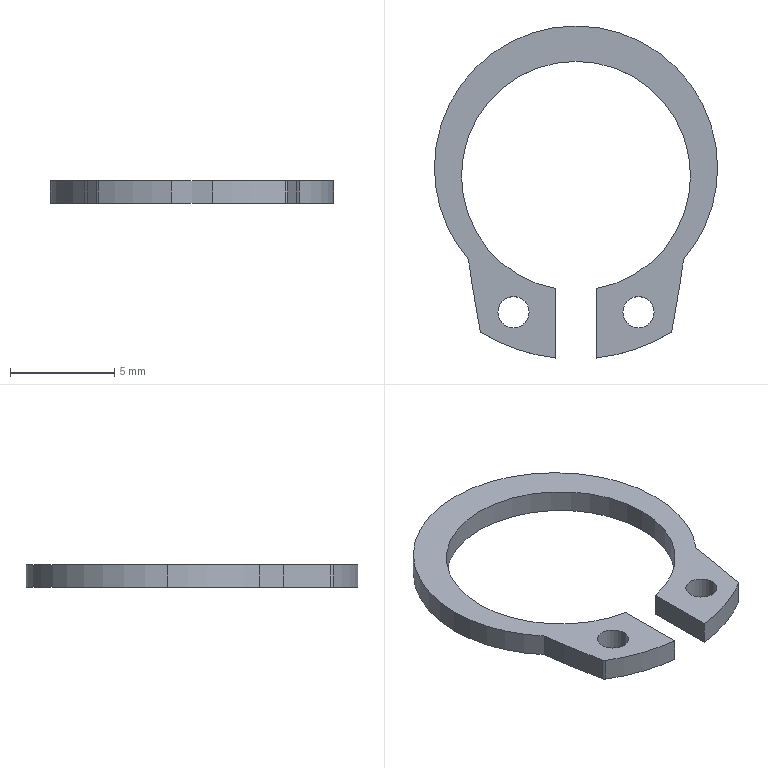Part | SolidWorks | features Extrusion 1 | 1 solid | 22 faces | box 13.6 x 15.943 x 1.1 mm | volume 71.659 mm3 | cylinder 14 | plane 8 | commonest cylinder face diameters 1.5 x4 11 x3 13.6 x3 0.4 x2 17.6 x2
STEP:
#1=CARTESIAN_POINT('',(2.25,-6.545,1.1));
#2=VERTEX_POINT('',#1);
#3=CARTESIAN_POINT('',(3.75,-6.545,1.1));
#4=VERTEX_POINT('',#3);
#5=CARTESIAN_POINT('',(3.,-6.545,1.1));
#6=DIRECTION('',(0.,0.,1.));
#7=DIRECTION('',(1.,0.,0.));
#8=AXIS2_PLACEMENT_3D('',#5,#6,#7);
#9=CIRCLE('',#8,0.75);
#10=EDGE_CURVE('',#2,#4,#9,.T.);
#11=ORIENTED_EDGE('',*,*,#10,.T.);
#12=CARTESIAN_POINT('',(3.75,-6.545,0.));
#13=VERTEX_POINT('',#12);
#14=CARTESIAN_POINT('',(3.75,-6.545,1.1));
#15=DIRECTION('',(0.,0.,-1.));
#16=VECTOR('',#15,1000.);
#17=LINE('',#14,#16);
#18=EDGE_CURVE('',#4,#13,#17,.T.);
#19=ORIENTED_EDGE('',*,*,#18,.T.);
#20=CARTESIAN_POINT('',(2.25,-6.545,0.));
#21=VERTEX_POINT('',#20);
#22=CARTESIAN_POINT('',(3.,-6.545,0.));
#23=DIRECTION('',(0.,0.,1.));
#24=DIRECTION('',(1.,0.,0.));
#25=AXIS2_PLACEMENT_3D('',#22,#23,#24);
#26=CIRCLE('',#25,0.75);
#27=EDGE_CURVE('',#21,#13,#26,.T.);
#28=ORIENTED_EDGE('',*,*,#27,.F.);
#29=CARTESIAN_POINT('',(2.25,-6.545,1.1));
#30=DIRECTION('',(0.,0.,-1.));
#31=VECTOR('',#30,1000.);
#32=LINE('',#29,#31);
#33=EDGE_CURVE('',#2,#21,#32,.T.);
#34=ORIENTED_EDGE('',*,*,#33,.F.);
#35=EDGE_LOOP('',(#11,#19,#28,#34));
#36=FACE_OUTER_BOUND('',#35,.T.);
#37=CARTESIAN_POINT('',(3.,-6.545,1.1));
#38=DIRECTION('',(0.,0.,-1.));
#39=DIRECTION('',(-1.,0.,0.));
#40=AXIS2_PLACEMENT_3D('',#37,#38,#39);
#41=CYLINDRICAL_SURFACE('',#40,0.75);
#42=ADVANCED_FACE('',(#36),#41,.F.);
#43=CARTESIAN_POINT('',(-3.75,-6.545,1.1));
#44=VERTEX_POINT('',#43);
#45=CARTESIAN_POINT('',(-2.25,-6.545,1.1));
#46=VERTEX_POINT('',#45);
#47=CARTESIAN_POINT('',(-3.,-6.545,1.1));
#48=DIRECTION('',(0.,0.,1.));
#49=DIRECTION('',(1.,0.,0.));
#50=AXIS2_PLACEMENT_3D('',#47,#48,#49);
#51=CIRCLE('',#50,0.75);
#52=EDGE_CURVE('',#44,#46,#51,.T.);
#53=ORIENTED_EDGE('',*,*,#52,.T.);
#54=CARTESIAN_POINT('',(-2.25,-6.545,0.));
#55=VERTEX_POINT('',#54);
#56=CARTESIAN_POINT('',(-2.25,-6.545,1.1));
#57=DIRECTION('',(0.,0.,-1.));
#58=VECTOR('',#57,1000.);
#59=LINE('',#56,#58);
#60=EDGE_CURVE('',#46,#55,#59,.T.);
#61=ORIENTED_EDGE('',*,*,#60,.T.);
#62=CARTESIAN_POINT('',(-3.75,-6.545,0.));
#63=VERTEX_POINT('',#62);
#64=CARTESIAN_POINT('',(-3.,-6.545,0.));
#65=DIRECTION('',(0.,0.,1.));
#66=DIRECTION('',(1.,0.,0.));
#67=AXIS2_PLACEMENT_3D('',#64,#65,#66);
#68=CIRCLE('',#67,0.75);
#69=EDGE_CURVE('',#63,#55,#68,.T.);
#70=ORIENTED_EDGE('',*,*,#69,.F.);
#71=CARTESIAN_POINT('',(-3.75,-6.545,1.1));
#72=DIRECTION('',(0.,0.,-1.));
#73=VECTOR('',#72,1000.);
#74=LINE('',#71,#73);
#75=EDGE_CURVE('',#44,#63,#74,.T.);
#76=ORIENTED_EDGE('',*,*,#75,.F.);
#77=EDGE_LOOP('',(#53,#61,#70,#76));
#78=FACE_OUTER_BOUND('',#77,.T.);
#79=CARTESIAN_POINT('',(-3.,-6.545,1.1));
#80=DIRECTION('',(0.,0.,-1.));
#81=DIRECTION('',(-1.,0.,0.));
#82=AXIS2_PLACEMENT_3D('',#79,#80,#81);
#83=CYLINDRICAL_SURFACE('',#82,0.75);
#84=ADVANCED_FACE('',(#78),#83,.F.);
#85=CARTESIAN_POINT('',(6.8,0.4,1.1));
#86=VERTEX_POINT('',#85);
#87=CARTESIAN_POINT('',(-6.8,0.4,1.1));
#88=VERTEX_POINT('',#87);
#89=CARTESIAN_POINT('',(0.,0.4,1.1));
#90=DIRECTION('',(0.,0.,1.));
#91=DIRECTION('',(1.,0.,0.));
#92=AXIS2_PLACEMENT_3D('',#89,#90,#91);
#93=CIRCLE('',#92,6.8);
#94=EDGE_CURVE('',#86,#88,#93,.T.);
#95=ORIENTED_EDGE('',*,*,#94,.F.);
#96=CARTESIAN_POINT('',(6.8,0.4,0.));
#97=VERTEX_POINT('',#96);
#98=CARTESIAN_POINT('',(6.8,0.4,1.1));
#99=DIRECTION('',(0.,0.,-1.));
#100=VECTOR('',#99,1000.);
#101=LINE('',#98,#100);
#102=EDGE_CURVE('',#86,#97,#101,.T.);
#103=ORIENTED_EDGE('',*,*,#102,.T.);
#104=CARTESIAN_POINT('',(-6.8,0.4,0.));
#105=VERTEX_POINT('',#104);
#106=CARTESIAN_POINT('',(0.,0.4,0.));
#107=DIRECTION('',(0.,0.,1.));
#108=DIRECTION('',(1.,0.,0.));
#109=AXIS2_PLACEMENT_3D('',#106,#107,#108);
#110=CIRCLE('',#109,6.8);
#111=EDGE_CURVE('',#97,#105,#110,.T.);
#112=ORIENTED_EDGE('',*,*,#111,.T.);
#113=CARTESIAN_POINT('',(-6.8,0.4,1.1));
#114=DIRECTION('',(0.,0.,-1.));
#115=VECTOR('',#114,1000.);
#116=LINE('',#113,#115);
#117=EDGE_CURVE('',#88,#105,#116,.T.);
#118=ORIENTED_EDGE('',*,*,#117,.F.);
#119=EDGE_LOOP('',(#95,#103,#112,#118));
#120=FACE_OUTER_BOUND('',#119,.T.);
#121=CARTESIAN_POINT('',(0.,0.4,1.1));
#122=DIRECTION('',(0.,0.,-1.));
#123=DIRECTION('',(-1.,0.,0.));
#124=AXIS2_PLACEMENT_3D('',#121,#122,#123);
#125=CYLINDRICAL_SURFACE('',#124,6.8);
#126=ADVANCED_FACE('',(#120),#125,.T.);
#127=CARTESIAN_POINT('',(-5.16,-4.028,1.1));
#128=VERTEX_POINT('',#127);
#129=CARTESIAN_POINT('',(0.,0.4,1.1));
#130=DIRECTION('',(0.,0.,1.));
#131=DIRECTION('',(1.,0.,0.));
#132=AXIS2_PLACEMENT_3D('',#129,#130,#131);
#133=CIRCLE('',#132,6.8);
#134=EDGE_CURVE('',#88,#128,#133,.T.);
#135=ORIENTED_EDGE('',*,*,#134,.F.);
#136=ORIENTED_EDGE('',*,*,#117,.T.);
#137=CARTESIAN_POINT('',(-5.16,-4.028,0.));
#138=VERTEX_POINT('',#137);
#139=CARTESIAN_POINT('',(0.,0.4,0.));
#140=DIRECTION('',(0.,0.,1.));
#141=DIRECTION('',(1.,0.,0.));
#142=AXIS2_PLACEMENT_3D('',#139,#140,#141);
#143=CIRCLE('',#142,6.8);
#144=EDGE_CURVE('',#105,#138,#143,.T.);
#145=ORIENTED_EDGE('',*,*,#144,.T.);
#146=CARTESIAN_POINT('',(-5.16,-4.028,1.1));
#147=DIRECTION('',(0.,0.,-1.));
#148=VECTOR('',#147,1000.);
#149=LINE('',#146,#148);
#150=EDGE_CURVE('',#128,#138,#149,.T.);
#151=ORIENTED_EDGE('',*,*,#150,.F.);
#152=EDGE_LOOP('',(#135,#136,#145,#151));
#153=FACE_OUTER_BOUND('',#152,.T.);
#154=CARTESIAN_POINT('',(0.,0.4,1.1));
#155=DIRECTION('',(0.,0.,-1.));
#156=DIRECTION('',(-1.,0.,0.));
#157=AXIS2_PLACEMENT_3D('',#154,#155,#156);
#158=CYLINDRICAL_SURFACE('',#157,6.8);
#159=ADVANCED_FACE('',(#153),#158,.T.);
#160=CARTESIAN_POINT('',(1.,-5.408,1.1));
#161=VERTEX_POINT('',#160);
#162=CARTESIAN_POINT('',(5.5,0.,1.1));
#163=VERTEX_POINT('',#162);
#164=CARTESIAN_POINT('',(0.,0.,1.1));
#165=DIRECTION('',(0.,0.,1.));
#166=DIRECTION('',(1.,0.,0.));
#167=AXIS2_PLACEMENT_3D('',#164,#165,#166);
#168=CIRCLE('',#167,5.5);
#169=EDGE_CURVE('',#161,#163,#168,.T.);
#170=ORIENTED_EDGE('',*,*,#169,.T.);
#171=CARTESIAN_POINT('',(5.5,0.,0.));
#172=VERTEX_POINT('',#171);
#173=CARTESIAN_POINT('',(5.5,0.,1.1));
#174=DIRECTION('',(0.,0.,-1.));
#175=VECTOR('',#174,1000.);
#176=LINE('',#173,#175);
#177=EDGE_CURVE('',#163,#172,#176,.T.);
#178=ORIENTED_EDGE('',*,*,#177,.T.);
#179=CARTESIAN_POINT('',(1.,-5.408,0.));
#180=VERTEX_POINT('',#179);
#181=CARTESIAN_POINT('',(0.,0.,0.));
#182=DIRECTION('',(0.,0.,1.));
#183=DIRECTION('',(1.,0.,0.));
#184=AXIS2_PLACEMENT_3D('',#181,#182,#183);
#185=CIRCLE('',#184,5.5);
#186=EDGE_CURVE('',#180,#172,#185,.T.);
#187=ORIENTED_EDGE('',*,*,#186,.F.);
#188=CARTESIAN_POINT('',(1.,-5.408,1.1));
#189=DIRECTION('',(0.,0.,-1.));
#190=VECTOR('',#189,1000.);
#191=LINE('',#188,#190);
#192=EDGE_CURVE('',#161,#180,#191,.T.);
#193=ORIENTED_EDGE('',*,*,#192,.F.);
#194=EDGE_LOOP('',(#170,#178,#187,#193));
#195=FACE_OUTER_BOUND('',#194,.T.);
#196=CARTESIAN_POINT('',(0.,0.,1.1));
#197=DIRECTION('',(0.,0.,-1.));
#198=DIRECTION('',(-1.,0.,0.));
#199=AXIS2_PLACEMENT_3D('',#196,#197,#198);
#200=CYLINDRICAL_SURFACE('',#199,5.5);
#201=ADVANCED_FACE('',(#195),#200,.F.);
#202=ORIENTED_EDGE('',*,*,#177,.F.);
#203=CARTESIAN_POINT('',(-5.5,0.,1.1));
#204=VERTEX_POINT('',#203);
#205=CARTESIAN_POINT('',(0.,0.,1.1));
#206=DIRECTION('',(0.,0.,1.));
#207=DIRECTION('',(1.,0.,0.));
#208=AXIS2_PLACEMENT_3D('',#205,#206,#207);
#209=CIRCLE('',#208,5.5);
#210=EDGE_CURVE('',#163,#204,#209,.T.);
#211=ORIENTED_EDGE('',*,*,#210,.T.);
#212=CARTESIAN_POINT('',(-5.5,0.,0.));
#213=VERTEX_POINT('',#212);
#214=CARTESIAN_POINT('',(-5.5,0.,1.1));
#215=DIRECTION('',(0.,0.,-1.));
#216=VECTOR('',#215,1000.);
#217=LINE('',#214,#216);
#218=EDGE_CURVE('',#204,#213,#217,.T.);
#219=ORIENTED_EDGE('',*,*,#218,.T.);
#220=CARTESIAN_POINT('',(0.,0.,0.));
#221=DIRECTION('',(0.,0.,1.));
#222=DIRECTION('',(1.,0.,0.));
#223=AXIS2_PLACEMENT_3D('',#220,#221,#222);
#224=CIRCLE('',#223,5.5);
#225=EDGE_CURVE('',#172,#213,#224,.T.);
#226=ORIENTED_EDGE('',*,*,#225,.F.);
#227=EDGE_LOOP('',(#202,#211,#219,#226));
#228=FACE_OUTER_BOUND('',#227,.T.);
#229=CARTESIAN_POINT('',(0.,0.,1.1));
#230=DIRECTION('',(0.,0.,-1.));
#231=DIRECTION('',(-1.,0.,0.));
#232=AXIS2_PLACEMENT_3D('',#229,#230,#231);
#233=CYLINDRICAL_SURFACE('',#232,5.5);
#234=ADVANCED_FACE('',(#228),#233,.F.);
#235=CARTESIAN_POINT('',(-4.511,-7.556,0.));
#236=VERTEX_POINT('',#235);
#237=CARTESIAN_POINT('',(-4.605,-7.419,0.));
#238=VERTEX_POINT('',#237);
#239=CARTESIAN_POINT('',(-4.408,-7.384,0.));
#240=DIRECTION('',(0.,0.,-1.));
#241=DIRECTION('',(1.,0.,0.));
#242=AXIS2_PLACEMENT_3D('',#239,#240,#241);
#243=CIRCLE('',#242,0.2);
#244=EDGE_CURVE('',#236,#238,#243,.T.);
#245=ORIENTED_EDGE('',*,*,#244,.F.);
#246=CARTESIAN_POINT('',(-4.511,-7.556,1.1));
#247=VERTEX_POINT('',#246);
#248=CARTESIAN_POINT('',(-4.511,-7.556,1.1));
#249=DIRECTION('',(0.,0.,-1.));
#250=VECTOR('',#249,1000.);
#251=LINE('',#248,#250);
#252=EDGE_CURVE('',#247,#236,#251,.T.);
#253=ORIENTED_EDGE('',*,*,#252,.F.);
#254=CARTESIAN_POINT('',(-4.605,-7.419,1.1));
#255=VERTEX_POINT('',#254);
#256=CARTESIAN_POINT('',(-4.408,-7.384,1.1));
#257=DIRECTION('',(0.,0.,-1.));
#258=DIRECTION('',(1.,0.,0.));
#259=AXIS2_PLACEMENT_3D('',#256,#257,#258);
#260=CIRCLE('',#259,0.2);
#261=EDGE_CURVE('',#247,#255,#260,.T.);
#262=ORIENTED_EDGE('',*,*,#261,.T.);
#263=CARTESIAN_POINT('',(-4.605,-7.419,1.1));
#264=DIRECTION('',(0.,0.,-1.));
#265=VECTOR('',#264,1000.);
#266=LINE('',#263,#265);
#267=EDGE_CURVE('',#255,#238,#266,.T.);
#268=ORIENTED_EDGE('',*,*,#267,.T.);
#269=EDGE_LOOP('',(#245,#253,#262,#268));
#270=FACE_OUTER_BOUND('',#269,.T.);
#271=CARTESIAN_POINT('',(-4.408,-7.384,1.1));
#272=DIRECTION('',(0.,0.,-1.));
#273=DIRECTION('',(-1.,0.,0.));
#274=AXIS2_PLACEMENT_3D('',#271,#272,#273);
#275=CYLINDRICAL_SURFACE('',#274,0.2);
#276=ADVANCED_FACE('',(#270),#275,.T.);
#277=CARTESIAN_POINT('',(-1.,-8.743,0.));
#278=VERTEX_POINT('',#277);
#279=CARTESIAN_POINT('',(0.,0.,0.));
#280=DIRECTION('',(0.,0.,1.));
#281=DIRECTION('',(1.,0.,0.));
#282=AXIS2_PLACEMENT_3D('',#279,#280,#281);
#283=CIRCLE('',#282,8.8);
#284=EDGE_CURVE('',#236,#278,#283,.T.);
#285=ORIENTED_EDGE('',*,*,#284,.T.);
#286=CARTESIAN_POINT('',(-1.,-8.743,1.1));
#287=VERTEX_POINT('',#286);
#288=CARTESIAN_POINT('',(-1.,-8.743,1.1));
#289=DIRECTION('',(0.,0.,-1.));
#290=VECTOR('',#289,1000.);
#291=LINE('',#288,#290);
#292=EDGE_CURVE('',#287,#278,#291,.T.);
#293=ORIENTED_EDGE('',*,*,#292,.F.);
#294=CARTESIAN_POINT('',(0.,0.,1.1));
#295=DIRECTION('',(0.,0.,1.));
#296=DIRECTION('',(1.,0.,0.));
#297=AXIS2_PLACEMENT_3D('',#294,#295,#296);
#298=CIRCLE('',#297,8.8);
#299=EDGE_CURVE('',#247,#287,#298,.T.);
#300=ORIENTED_EDGE('',*,*,#299,.F.);
#301=ORIENTED_EDGE('',*,*,#252,.T.);
#302=EDGE_LOOP('',(#285,#293,#300,#301));
#303=FACE_OUTER_BOUND('',#302,.T.);
#304=CARTESIAN_POINT('',(0.,0.,1.1));
#305=DIRECTION('',(0.,0.,-1.));
#306=DIRECTION('',(-1.,0.,0.));
#307=AXIS2_PLACEMENT_3D('',#304,#305,#306);
#308=CYLINDRICAL_SURFACE('',#307,8.8);
#309=ADVANCED_FACE('',(#303),#308,.T.);
#310=CARTESIAN_POINT('',(-1.,-5.408,0.));
#311=VERTEX_POINT('',#310);
#312=CARTESIAN_POINT('',(-1.,0.,0.));
#313=DIRECTION('',(0.,-1.,0.));
#314=VECTOR('',#313,1000.);
#315=LINE('',#312,#314);
#316=EDGE_CURVE('',#311,#278,#315,.T.);
#317=ORIENTED_EDGE('',*,*,#316,.F.);
#318=CARTESIAN_POINT('',(-1.,-5.408,1.1));
#319=VERTEX_POINT('',#318);
#320=CARTESIAN_POINT('',(-1.,-5.408,1.1));
#321=DIRECTION('',(0.,0.,-1.));
#322=VECTOR('',#321,1000.);
#323=LINE('',#320,#322);
#324=EDGE_CURVE('',#319,#311,#323,.T.);
#325=ORIENTED_EDGE('',*,*,#324,.F.);
#326=CARTESIAN_POINT('',(-1.,0.,1.1));
#327=DIRECTION('',(0.,-1.,0.));
#328=VECTOR('',#327,1000.);
#329=LINE('',#326,#328);
#330=EDGE_CURVE('',#319,#287,#329,.T.);
#331=ORIENTED_EDGE('',*,*,#330,.T.);
#332=ORIENTED_EDGE('',*,*,#292,.T.);
#333=EDGE_LOOP('',(#317,#325,#331,#332));
#334=FACE_OUTER_BOUND('',#333,.T.);
#335=CARTESIAN_POINT('',(-1.,0.,1.1));
#336=DIRECTION('',(1.,0.,0.));
#337=DIRECTION('',(0.,1.,0.));
#338=AXIS2_PLACEMENT_3D('',#335,#336,#337);
#339=PLANE('',#338);
#340=ADVANCED_FACE('',(#334),#339,.T.);
#341=ORIENTED_EDGE('',*,*,#218,.F.);
#342=CARTESIAN_POINT('',(0.,0.,1.1));
#343=DIRECTION('',(0.,0.,1.));
#344=DIRECTION('',(1.,0.,0.));
#345=AXIS2_PLACEMENT_3D('',#342,#343,#344);
#346=CIRCLE('',#345,5.5);
#347=EDGE_CURVE('',#204,#319,#346,.T.);
#348=ORIENTED_EDGE('',*,*,#347,.T.);
#349=ORIENTED_EDGE('',*,*,#324,.T.);
#350=CARTESIAN_POINT('',(0.,0.,0.));
#351=DIRECTION('',(0.,0.,1.));
#352=DIRECTION('',(1.,0.,0.));
#353=AXIS2_PLACEMENT_3D('',#350,#351,#352);
#354=CIRCLE('',#353,5.5);
#355=EDGE_CURVE('',#213,#311,#354,.T.);
#356=ORIENTED_EDGE('',*,*,#355,.F.);
#357=EDGE_LOOP('',(#341,#348,#349,#356));
#358=FACE_OUTER_BOUND('',#357,.T.);
#359=CARTESIAN_POINT('',(0.,0.,1.1));
#360=DIRECTION('',(0.,0.,-1.));
#361=DIRECTION('',(-1.,0.,0.));
#362=AXIS2_PLACEMENT_3D('',#359,#360,#361);
#363=CYLINDRICAL_SURFACE('',#362,5.5);
#364=ADVANCED_FACE('',(#358),#363,.F.);
#365=CARTESIAN_POINT('',(1.,-8.743,0.));
#366=VERTEX_POINT('',#365);
#367=CARTESIAN_POINT('',(1.,0.,0.));
#368=DIRECTION('',(0.,1.,0.));
#369=VECTOR('',#368,1000.);
#370=LINE('',#367,#369);
#371=EDGE_CURVE('',#366,#180,#370,.T.);
#372=ORIENTED_EDGE('',*,*,#371,.F.);
#373=CARTESIAN_POINT('',(1.,-8.743,1.1));
#374=VERTEX_POINT('',#373);
#375=CARTESIAN_POINT('',(1.,-8.743,1.1));
#376=DIRECTION('',(0.,0.,-1.));
#377=VECTOR('',#376,1000.);
#378=LINE('',#375,#377);
#379=EDGE_CURVE('',#374,#366,#378,.T.);
#380=ORIENTED_EDGE('',*,*,#379,.F.);
#381=CARTESIAN_POINT('',(1.,0.,1.1));
#382=DIRECTION('',(0.,1.,0.));
#383=VECTOR('',#382,1000.);
#384=LINE('',#381,#383);
#385=EDGE_CURVE('',#374,#161,#384,.T.);
#386=ORIENTED_EDGE('',*,*,#385,.T.);
#387=ORIENTED_EDGE('',*,*,#192,.T.);
#388=EDGE_LOOP('',(#372,#380,#386,#387));
#389=FACE_OUTER_BOUND('',#388,.T.);
#390=CARTESIAN_POINT('',(1.,0.,1.1));
#391=DIRECTION('',(-1.,0.,0.));
#392=DIRECTION('',(0.,0.,1.));
#393=AXIS2_PLACEMENT_3D('',#390,#391,#392);
#394=PLANE('',#393);
#395=ADVANCED_FACE('',(#389),#394,.T.);
#396=CARTESIAN_POINT('',(4.511,-7.556,0.));
#397=VERTEX_POINT('',#396);
#398=CARTESIAN_POINT('',(0.,0.,0.));
#399=DIRECTION('',(0.,0.,1.));
#400=DIRECTION('',(1.,0.,0.));
#401=AXIS2_PLACEMENT_3D('',#398,#399,#400);
#402=CIRCLE('',#401,8.8);
#403=EDGE_CURVE('',#366,#397,#402,.T.);
#404=ORIENTED_EDGE('',*,*,#403,.T.);
#405=CARTESIAN_POINT('',(4.511,-7.556,1.1));
#406=VERTEX_POINT('',#405);
#407=CARTESIAN_POINT('',(4.511,-7.556,1.1));
#408=DIRECTION('',(0.,0.,-1.));
#409=VECTOR('',#408,1000.);
#410=LINE('',#407,#409);
#411=EDGE_CURVE('',#406,#397,#410,.T.);
#412=ORIENTED_EDGE('',*,*,#411,.F.);
#413=CARTESIAN_POINT('',(0.,0.,1.1));
#414=DIRECTION('',(0.,0.,1.));
#415=DIRECTION('',(1.,0.,0.));
#416=AXIS2_PLACEMENT_3D('',#413,#414,#415);
#417=CIRCLE('',#416,8.8);
#418=EDGE_CURVE('',#374,#406,#417,.T.);
#419=ORIENTED_EDGE('',*,*,#418,.F.);
#420=ORIENTED_EDGE('',*,*,#379,.T.);
#421=EDGE_LOOP('',(#404,#412,#419,#420));
#422=FACE_OUTER_BOUND('',#421,.T.);
#423=CARTESIAN_POINT('',(0.,0.,1.1));
#424=DIRECTION('',(0.,0.,-1.));
#425=DIRECTION('',(-1.,0.,0.));
#426=AXIS2_PLACEMENT_3D('',#423,#424,#425);
#427=CYLINDRICAL_SURFACE('',#426,8.8);
#428=ADVANCED_FACE('',(#422),#427,.T.);
#429=CARTESIAN_POINT('',(4.605,-7.419,0.));
#430=VERTEX_POINT('',#429);
#431=CARTESIAN_POINT('',(4.408,-7.384,0.));
#432=DIRECTION('',(0.,0.,1.));
#433=DIRECTION('',(1.,0.,0.));
#434=AXIS2_PLACEMENT_3D('',#431,#432,#433);
#435=CIRCLE('',#434,0.2);
#436=EDGE_CURVE('',#397,#430,#435,.T.);
#437=ORIENTED_EDGE('',*,*,#436,.T.);
#438=CARTESIAN_POINT('',(4.605,-7.419,1.1));
#439=VERTEX_POINT('',#438);
#440=CARTESIAN_POINT('',(4.605,-7.419,1.1));
#441=DIRECTION('',(0.,0.,-1.));
#442=VECTOR('',#441,1000.);
#443=LINE('',#440,#442);
#444=EDGE_CURVE('',#439,#430,#443,.T.);
#445=ORIENTED_EDGE('',*,*,#444,.F.);
#446=CARTESIAN_POINT('',(4.408,-7.384,1.1));
#447=DIRECTION('',(0.,0.,1.));
#448=DIRECTION('',(1.,0.,0.));
#449=AXIS2_PLACEMENT_3D('',#446,#447,#448);
#450=CIRCLE('',#449,0.2);
#451=EDGE_CURVE('',#406,#439,#450,.T.);
#452=ORIENTED_EDGE('',*,*,#451,.F.);
#453=ORIENTED_EDGE('',*,*,#411,.T.);
#454=EDGE_LOOP('',(#437,#445,#452,#453));
#455=FACE_OUTER_BOUND('',#454,.T.);
#456=CARTESIAN_POINT('',(4.408,-7.384,1.1));
#457=DIRECTION('',(0.,0.,-1.));
#458=DIRECTION('',(-1.,0.,0.));
#459=AXIS2_PLACEMENT_3D('',#456,#457,#458);
#460=CYLINDRICAL_SURFACE('',#459,0.2);
#461=ADVANCED_FACE('',(#455),#460,.T.);
#462=CARTESIAN_POINT('',(5.,-5.181,0.));
#463=VERTEX_POINT('',#462);
#464=CARTESIAN_POINT('',(5.735,-1.011,0.));
#465=DIRECTION('',(-0.1736,-0.9848,0.));
#466=VECTOR('',#465,1000.);
#467=LINE('',#464,#466);
#468=EDGE_CURVE('',#463,#430,#467,.T.);
#469=ORIENTED_EDGE('',*,*,#468,.F.);
#470=CARTESIAN_POINT('',(5.,-5.181,1.1));
#471=VERTEX_POINT('',#470);
#472=CARTESIAN_POINT('',(5.,-5.181,1.1));
#473=DIRECTION('',(0.,0.,-1.));
#474=VECTOR('',#473,1000.);
#475=LINE('',#472,#474);
#476=EDGE_CURVE('',#471,#463,#475,.T.);
#477=ORIENTED_EDGE('',*,*,#476,.F.);
#478=CARTESIAN_POINT('',(5.735,-1.011,1.1));
#479=DIRECTION('',(-0.1736,-0.9848,0.));
#480=VECTOR('',#479,1000.);
#481=LINE('',#478,#480);
#482=EDGE_CURVE('',#471,#439,#481,.T.);
#483=ORIENTED_EDGE('',*,*,#482,.T.);
#484=ORIENTED_EDGE('',*,*,#444,.T.);
#485=EDGE_LOOP('',(#469,#477,#483,#484));
#486=FACE_OUTER_BOUND('',#485,.T.);
#487=CARTESIAN_POINT('',(5.735,-1.011,1.1));
#488=DIRECTION('',(0.9848,-0.1736,0.));
#489=DIRECTION('',(0.1736,0.9848,0.));
#490=AXIS2_PLACEMENT_3D('',#487,#488,#489);
#491=PLANE('',#490);
#492=ADVANCED_FACE('',(#486),#491,.T.);
#493=CARTESIAN_POINT('',(5.16,-4.028,0.));
#494=VERTEX_POINT('',#493);
#495=CARTESIAN_POINT('',(5.613,-0.7814,0.));
#496=DIRECTION('',(0.1379,0.9904,0.));
#497=VECTOR('',#496,1000.);
#498=LINE('',#495,#497);
#499=EDGE_CURVE('',#463,#494,#498,.T.);
#500=ORIENTED_EDGE('',*,*,#499,.T.);
#501=CARTESIAN_POINT('',(5.16,-4.028,1.1));
#502=VERTEX_POINT('',#501);
#503=CARTESIAN_POINT('',(5.16,-4.028,1.1));
#504=DIRECTION('',(0.,0.,-1.));
#505=VECTOR('',#504,1000.);
#506=LINE('',#503,#505);
#507=EDGE_CURVE('',#502,#494,#506,.T.);
#508=ORIENTED_EDGE('',*,*,#507,.F.);
#509=CARTESIAN_POINT('',(5.613,-0.7814,1.1));
#510=DIRECTION('',(0.1379,0.9904,0.));
#511=VECTOR('',#510,1000.);
#512=LINE('',#509,#511);
#513=EDGE_CURVE('',#471,#502,#512,.T.);
#514=ORIENTED_EDGE('',*,*,#513,.F.);
#515=ORIENTED_EDGE('',*,*,#476,.T.);
#516=EDGE_LOOP('',(#500,#508,#514,#515));
#517=FACE_OUTER_BOUND('',#516,.T.);
#518=CARTESIAN_POINT('',(5.613,-0.7814,1.1));
#519=DIRECTION('',(-0.9904,0.1379,0.));
#520=DIRECTION('',(-0.1379,-0.9904,0.));
#521=AXIS2_PLACEMENT_3D('',#518,#519,#520);
#522=PLANE('',#521);
#523=ADVANCED_FACE('',(#517),#522,.F.);
#524=ORIENTED_EDGE('',*,*,#102,.F.);
#525=CARTESIAN_POINT('',(0.,0.4,1.1));
#526=DIRECTION('',(0.,0.,1.));
#527=DIRECTION('',(1.,0.,0.));
#528=AXIS2_PLACEMENT_3D('',#525,#526,#527);
#529=CIRCLE('',#528,6.8);
#530=EDGE_CURVE('',#502,#86,#529,.T.);
#531=ORIENTED_EDGE('',*,*,#530,.F.);
#532=ORIENTED_EDGE('',*,*,#507,.T.);
#533=CARTESIAN_POINT('',(0.,0.4,0.));
#534=DIRECTION('',(0.,0.,1.));
#535=DIRECTION('',(1.,0.,0.));
#536=AXIS2_PLACEMENT_3D('',#533,#534,#535);
#537=CIRCLE('',#536,6.8);
#538=EDGE_CURVE('',#494,#97,#537,.T.);
#539=ORIENTED_EDGE('',*,*,#538,.T.);
#540=EDGE_LOOP('',(#524,#531,#532,#539));
#541=FACE_OUTER_BOUND('',#540,.T.);
#542=CARTESIAN_POINT('',(0.,0.4,1.1));
#543=DIRECTION('',(0.,0.,-1.));
#544=DIRECTION('',(-1.,0.,0.));
#545=AXIS2_PLACEMENT_3D('',#542,#543,#544);
#546=CYLINDRICAL_SURFACE('',#545,6.8);
#547=ADVANCED_FACE('',(#541),#546,.T.);
#548=CARTESIAN_POINT('',(-5.,-5.181,0.));
#549=VERTEX_POINT('',#548);
#550=CARTESIAN_POINT('',(-5.613,-0.7814,0.));
#551=DIRECTION('',(-0.1379,0.9904,0.));
#552=VECTOR('',#551,1000.);
#553=LINE('',#550,#552);
#554=EDGE_CURVE('',#549,#138,#553,.T.);
#555=ORIENTED_EDGE('',*,*,#554,.F.);
#556=CARTESIAN_POINT('',(-5.,-5.181,1.1));
#557=VERTEX_POINT('',#556);
#558=CARTESIAN_POINT('',(-5.,-5.181,1.1));
#559=DIRECTION('',(0.,0.,-1.));
#560=VECTOR('',#559,1000.);
#561=LINE('',#558,#560);
#562=EDGE_CURVE('',#557,#549,#561,.T.);
#563=ORIENTED_EDGE('',*,*,#562,.F.);
#564=CARTESIAN_POINT('',(-5.613,-0.7814,1.1));
#565=DIRECTION('',(-0.1379,0.9904,0.));
#566=VECTOR('',#565,1000.);
#567=LINE('',#564,#566);
#568=EDGE_CURVE('',#557,#128,#567,.T.);
#569=ORIENTED_EDGE('',*,*,#568,.T.);
#570=ORIENTED_EDGE('',*,*,#150,.T.);
#571=EDGE_LOOP('',(#555,#563,#569,#570));
#572=FACE_OUTER_BOUND('',#571,.T.);
#573=CARTESIAN_POINT('',(-5.613,-0.7814,1.1));
#574=DIRECTION('',(-0.9904,-0.1379,0.));
#575=DIRECTION('',(0.1379,-0.9904,0.));
#576=AXIS2_PLACEMENT_3D('',#573,#574,#575);
#577=PLANE('',#576);
#578=ADVANCED_FACE('',(#572),#577,.T.);
#579=ORIENTED_EDGE('',*,*,#60,.F.);
#580=CARTESIAN_POINT('',(-3.,-6.545,1.1));
#581=DIRECTION('',(0.,0.,1.));
#582=DIRECTION('',(1.,0.,0.));
#583=AXIS2_PLACEMENT_3D('',#580,#581,#582);
#584=CIRCLE('',#583,0.75);
#585=EDGE_CURVE('',#46,#44,#584,.T.);
#586=ORIENTED_EDGE('',*,*,#585,.T.);
#587=ORIENTED_EDGE('',*,*,#75,.T.);
#588=CARTESIAN_POINT('',(-3.,-6.545,0.));
#589=DIRECTION('',(0.,0.,1.));
#590=DIRECTION('',(1.,0.,0.));
#591=AXIS2_PLACEMENT_3D('',#588,#589,#590);
#592=CIRCLE('',#591,0.75);
#593=EDGE_CURVE('',#55,#63,#592,.T.);
#594=ORIENTED_EDGE('',*,*,#593,.F.);
#595=EDGE_LOOP('',(#579,#586,#587,#594));
#596=FACE_OUTER_BOUND('',#595,.T.);
#597=CARTESIAN_POINT('',(-3.,-6.545,1.1));
#598=DIRECTION('',(0.,0.,-1.));
#599=DIRECTION('',(-1.,0.,0.));
#600=AXIS2_PLACEMENT_3D('',#597,#598,#599);
#601=CYLINDRICAL_SURFACE('',#600,0.75);
#602=ADVANCED_FACE('',(#596),#601,.F.);
#603=ORIENTED_EDGE('',*,*,#18,.F.);
#604=CARTESIAN_POINT('',(3.,-6.545,1.1));
#605=DIRECTION('',(0.,0.,1.));
#606=DIRECTION('',(1.,0.,0.));
#607=AXIS2_PLACEMENT_3D('',#604,#605,#606);
#608=CIRCLE('',#607,0.75);
#609=EDGE_CURVE('',#4,#2,#608,.T.);
#610=ORIENTED_EDGE('',*,*,#609,.T.);
#611=ORIENTED_EDGE('',*,*,#33,.T.);
#612=CARTESIAN_POINT('',(3.,-6.545,0.));
#613=DIRECTION('',(0.,0.,1.));
#614=DIRECTION('',(1.,0.,0.));
#615=AXIS2_PLACEMENT_3D('',#612,#613,#614);
#616=CIRCLE('',#615,0.75);
#617=EDGE_CURVE('',#13,#21,#616,.T.);
#618=ORIENTED_EDGE('',*,*,#617,.F.);
#619=EDGE_LOOP('',(#603,#610,#611,#618));
#620=FACE_OUTER_BOUND('',#619,.T.);
#621=CARTESIAN_POINT('',(3.,-6.545,1.1));
#622=DIRECTION('',(0.,0.,-1.));
#623=DIRECTION('',(-1.,0.,0.));
#624=AXIS2_PLACEMENT_3D('',#621,#622,#623);
#625=CYLINDRICAL_SURFACE('',#624,0.75);
#626=ADVANCED_FACE('',(#620),#625,.F.);
#627=CARTESIAN_POINT('',(-5.735,-1.011,0.));
#628=DIRECTION('',(0.1736,-0.9848,0.));
#629=VECTOR('',#628,1000.);
#630=LINE('',#627,#629);
#631=EDGE_CURVE('',#549,#238,#630,.T.);
#632=ORIENTED_EDGE('',*,*,#631,.T.);
#633=ORIENTED_EDGE('',*,*,#267,.F.);
#634=CARTESIAN_POINT('',(-5.735,-1.011,1.1));
#635=DIRECTION('',(0.1736,-0.9848,0.));
#636=VECTOR('',#635,1000.);
#637=LINE('',#634,#636);
#638=EDGE_CURVE('',#557,#255,#637,.T.);
#639=ORIENTED_EDGE('',*,*,#638,.F.);
#640=ORIENTED_EDGE('',*,*,#562,.T.);
#641=EDGE_LOOP('',(#632,#633,#639,#640));
#642=FACE_OUTER_BOUND('',#641,.T.);
#643=CARTESIAN_POINT('',(-5.735,-1.011,1.1));
#644=DIRECTION('',(0.9848,0.1736,0.));
#645=DIRECTION('',(-0.1736,0.9848,0.));
#646=AXIS2_PLACEMENT_3D('',#643,#644,#645);
#647=PLANE('',#646);
#648=ADVANCED_FACE('',(#642),#647,.F.);
#649=ORIENTED_EDGE('',*,*,#10,.F.);
#650=ORIENTED_EDGE('',*,*,#609,.F.);
#651=EDGE_LOOP('',(#649,#650));
#652=FACE_BOUND('',#651,.T.);
#653=ORIENTED_EDGE('',*,*,#52,.F.);
#654=ORIENTED_EDGE('',*,*,#585,.F.);
#655=EDGE_LOOP('',(#653,#654));
#656=FACE_BOUND('',#655,.T.);
#657=ORIENTED_EDGE('',*,*,#261,.F.);
#658=ORIENTED_EDGE('',*,*,#299,.T.);
#659=ORIENTED_EDGE('',*,*,#330,.F.);
#660=ORIENTED_EDGE('',*,*,#347,.F.);
#661=ORIENTED_EDGE('',*,*,#210,.F.);
#662=ORIENTED_EDGE('',*,*,#169,.F.);
#663=ORIENTED_EDGE('',*,*,#385,.F.);
#664=ORIENTED_EDGE('',*,*,#418,.T.);
#665=ORIENTED_EDGE('',*,*,#451,.T.);
#666=ORIENTED_EDGE('',*,*,#482,.F.);
#667=ORIENTED_EDGE('',*,*,#513,.T.);
#668=ORIENTED_EDGE('',*,*,#530,.T.);
#669=ORIENTED_EDGE('',*,*,#94,.T.);
#670=ORIENTED_EDGE('',*,*,#134,.T.);
#671=ORIENTED_EDGE('',*,*,#568,.F.);
#672=ORIENTED_EDGE('',*,*,#638,.T.);
#673=EDGE_LOOP('',(#657,#658,#659,#660,#661,#662,#663,#664,#665,#666,#667,#668,#669,#670,#671,#672));
#674=FACE_OUTER_BOUND('',#673,.T.);
#675=CARTESIAN_POINT('',(0.,0.,1.1));
#676=DIRECTION('',(0.,0.,1.));
#677=DIRECTION('',(1.,0.,0.));
#678=AXIS2_PLACEMENT_3D('',#675,#676,#677);
#679=PLANE('',#678);
#680=ADVANCED_FACE('',(#652,#656,#674),#679,.T.);
#681=ORIENTED_EDGE('',*,*,#27,.T.);
#682=ORIENTED_EDGE('',*,*,#617,.T.);
#683=EDGE_LOOP('',(#681,#682));
#684=FACE_BOUND('',#683,.T.);
#685=ORIENTED_EDGE('',*,*,#69,.T.);
#686=ORIENTED_EDGE('',*,*,#593,.T.);
#687=EDGE_LOOP('',(#685,#686));
#688=FACE_BOUND('',#687,.T.);
#689=ORIENTED_EDGE('',*,*,#244,.T.);
#690=ORIENTED_EDGE('',*,*,#631,.F.);
#691=ORIENTED_EDGE('',*,*,#554,.T.);
#692=ORIENTED_EDGE('',*,*,#144,.F.);
#693=ORIENTED_EDGE('',*,*,#111,.F.);
#694=ORIENTED_EDGE('',*,*,#538,.F.);
#695=ORIENTED_EDGE('',*,*,#499,.F.);
#696=ORIENTED_EDGE('',*,*,#468,.T.);
#697=ORIENTED_EDGE('',*,*,#436,.F.);
#698=ORIENTED_EDGE('',*,*,#403,.F.);
#699=ORIENTED_EDGE('',*,*,#371,.T.);
#700=ORIENTED_EDGE('',*,*,#186,.T.);
#701=ORIENTED_EDGE('',*,*,#225,.T.);
#702=ORIENTED_EDGE('',*,*,#355,.T.);
#703=ORIENTED_EDGE('',*,*,#316,.T.);
#704=ORIENTED_EDGE('',*,*,#284,.F.);
#705=EDGE_LOOP('',(#689,#690,#691,#692,#693,#694,#695,#696,#697,#698,#699,#700,#701,#702,#703,#704));
#706=FACE_OUTER_BOUND('',#705,.T.);
#707=CARTESIAN_POINT('',(0.,0.,0.));
#708=DIRECTION('',(0.,0.,1.));
#709=DIRECTION('',(1.,0.,0.));
#710=AXIS2_PLACEMENT_3D('',#707,#708,#709);
#711=PLANE('',#710);
#712=ADVANCED_FACE('',(#684,#688,#706),#711,.F.);
#713=CLOSED_SHELL('',(#42,#84,#126,#159,#201,#234,#276,#309,#340,#364,#395,#428,#461,#492,#523,#547,#578,#602,#626,#648,#680,#712));
#714=MANIFOLD_SOLID_BREP('',#713);
#715=CARTESIAN_POINT('',(0.,0.,0.));
#716=DIRECTION('',(0.,0.,1.));
#717=DIRECTION('',(1.,0.,0.));
#718=AXIS2_PLACEMENT_3D('',#715,#716,#717);
#719=(LENGTH_UNIT()NAMED_UNIT(*)SI_UNIT(.MILLI.,.METRE.));
#720=UNCERTAINTY_MEASURE_WITH_UNIT(LENGTH_MEASURE(0.00001),#719,'','');
#721=(NAMED_UNIT(*)PLANE_ANGLE_UNIT()SI_UNIT($,.RADIAN.));
#722=(NAMED_UNIT(*)SI_UNIT($,.STERADIAN.)SOLID_ANGLE_UNIT());
#723=(GEOMETRIC_REPRESENTATION_CONTEXT(3)GLOBAL_UNCERTAINTY_ASSIGNED_CONTEXT((#720))GLOBAL_UNIT_ASSIGNED_CONTEXT((#719,#721,#722))REPRESENTATION_CONTEXT('',''));
#724=ADVANCED_BREP_SHAPE_REPRESENTATION('',(#714,#718),#723);